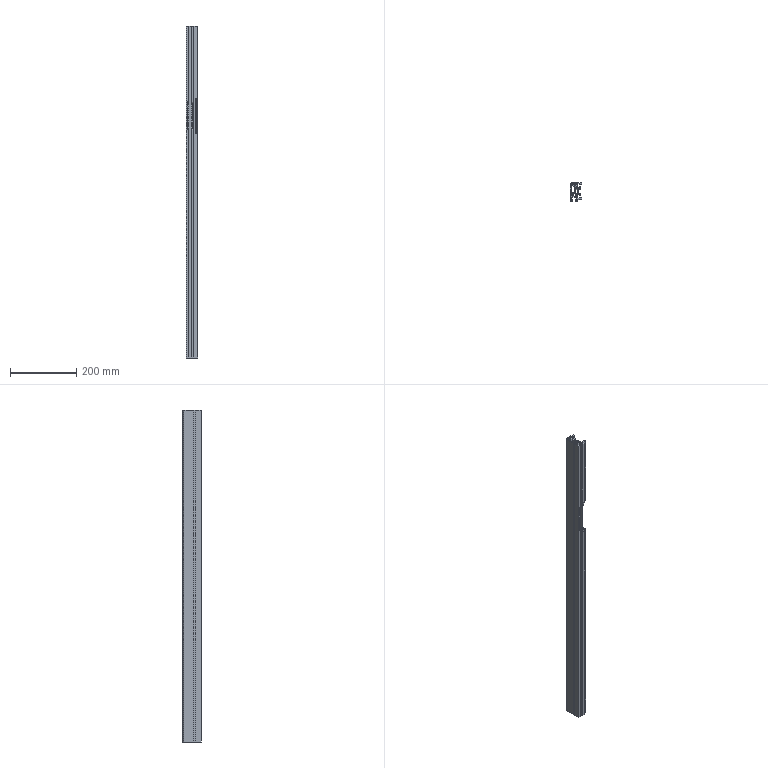Part | STEP file | 1 solid | 184 faces | box 35 x 55 x 1000 mm | volume 771122 mm3 | plane 134 | cylinder 41 | cone 9 | commonest cylinder face diameters 2.5 x9 2 x8 6.5 x6 2.3 x4 10 x4 11 x4